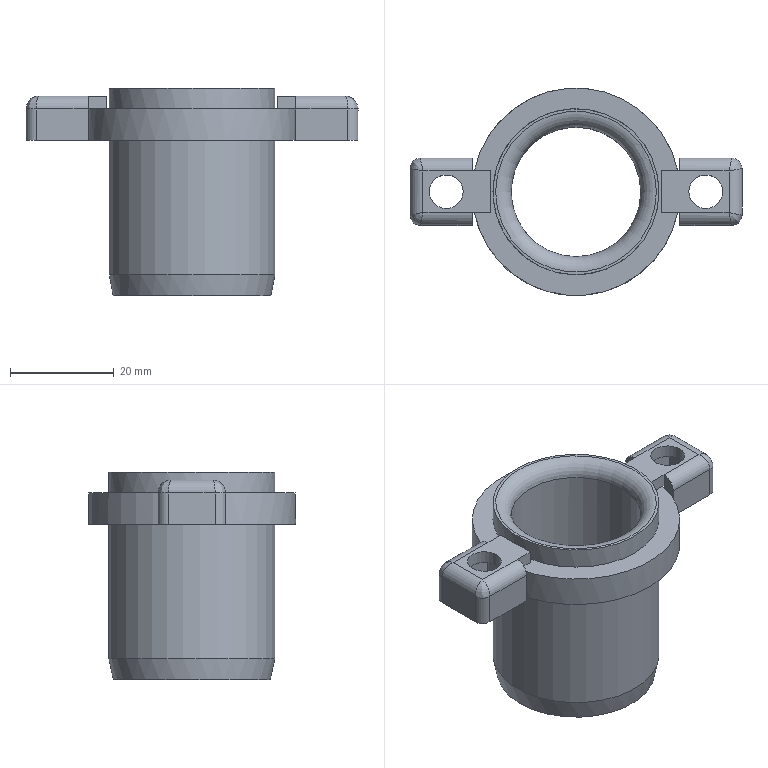Part | STEP file | gslz 2016.10.28-6_id442_x_t | 1 solid | 54 faces | box 64 x 40 x 40 mm | volume 16525 mm3 | plane 32 | cylinder 16 | spline 4 | torus 1 | cone 1 | commonest cylinder face diameters 5 x6 4 x4 6.5 x2 32 x2 25 x1 40 x1